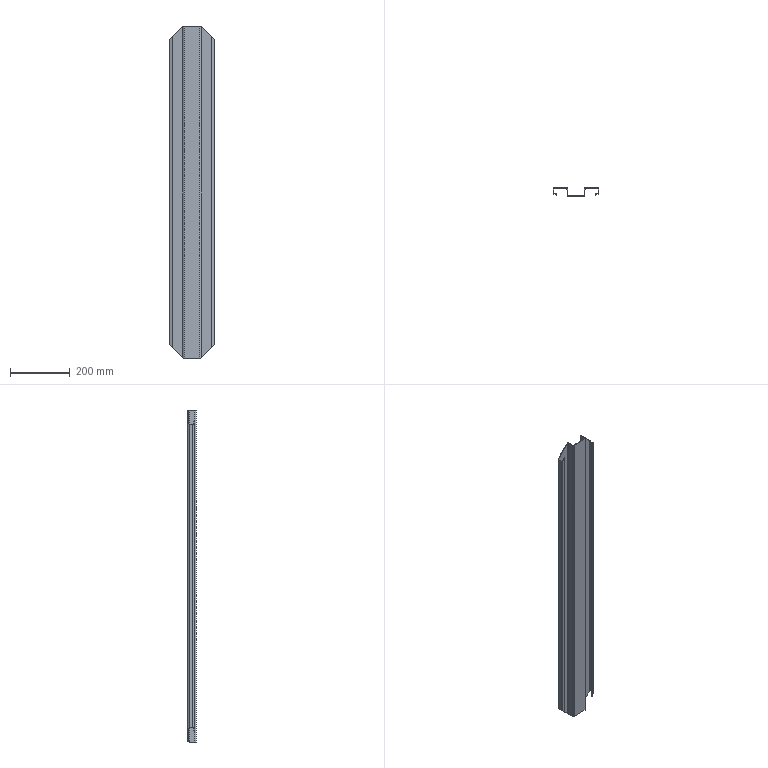Part | STEP file | 750038184 | 1 solid | 62 faces | box 154 x 27 x 1113 mm | volume 542434 mm3 | plane 34 | cylinder 16 | spline 12 | commonest cylinder face diameters 4 x8 8 x8